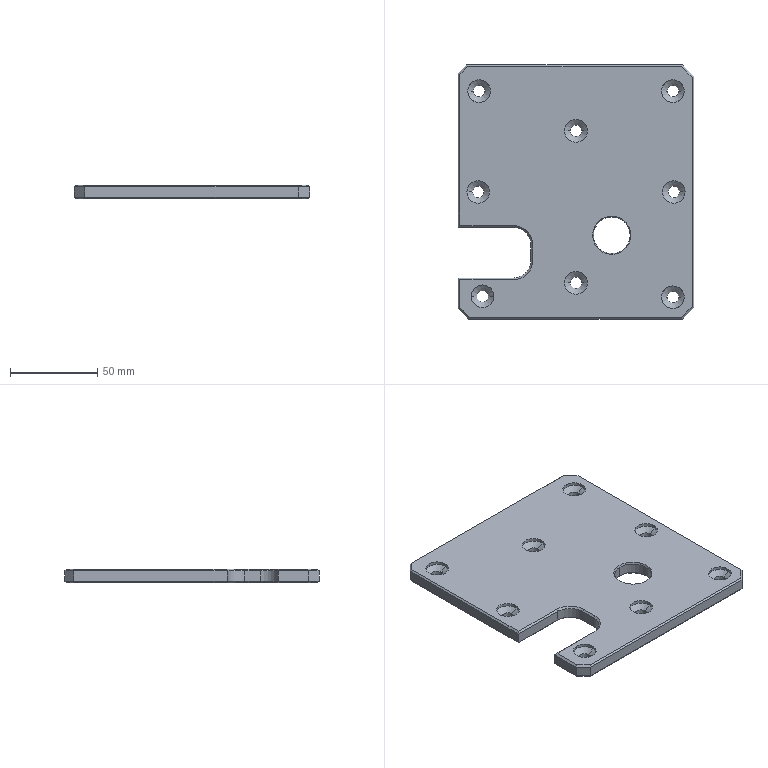Part | Creo | 1 solid | 100 faces | box 135 x 145.5 x 8 mm | volume 139312 mm3 | plane 40 | cylinder 36 | cone 24 | commonest cylinder face diameters 6.6 x16 13 x16 20 x2 21 x2